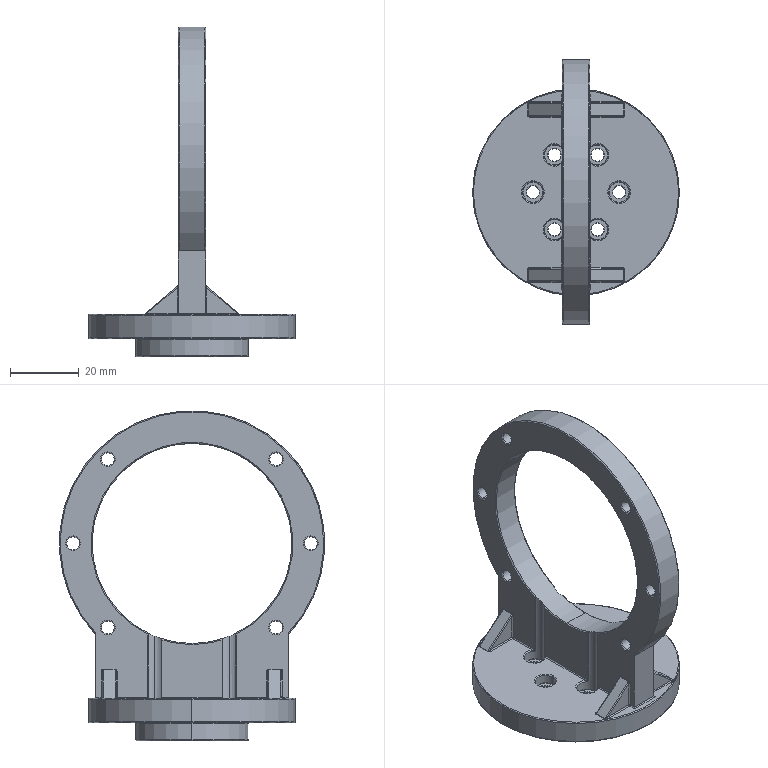Part | SolidWorks | features ICE 6, Fillet 2, Extrusion 1, MirrorPattern 1 | 1 solid | 282 faces | box 60 x 77 x 95.8 mm | volume 43529 mm3 | torus 110 | cylinder 107 | plane 33 | spline 24 | sphere 8 | commonest cylinder face diameters 0.6 x52 3.7 x24 6 x24 32.8 x2 58 x2 60 x2